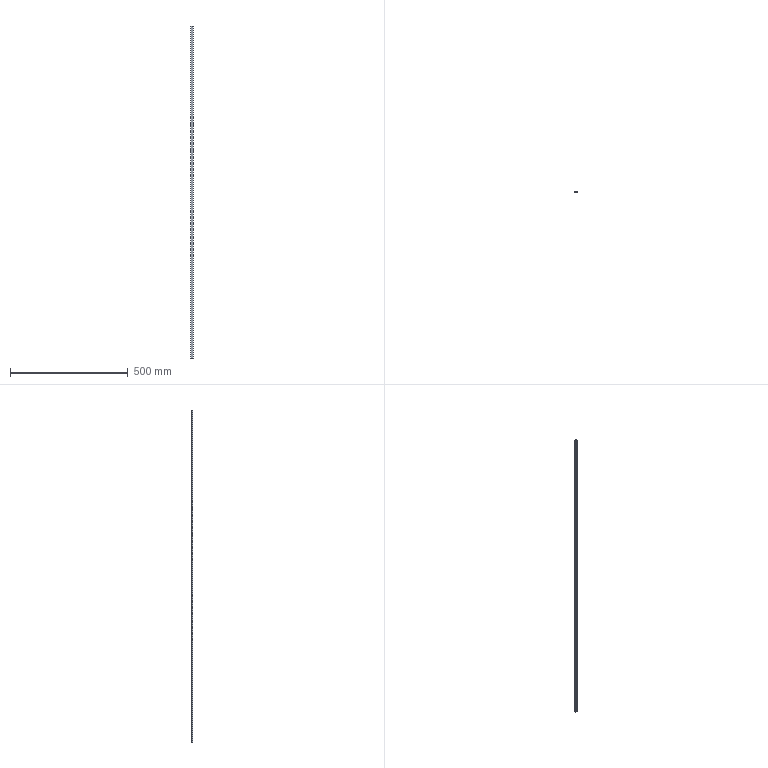Part | SolidWorks | features Extrusion 1 | 1 solid | 20 faces | box 10 x 6 x 1410 mm | volume 19879 mm3 | plane 12 | cylinder 8 | commonest cylinder face diameters 1 x3 2 x3 11.891 x1 12.891 x1
STEP:
#1=CARTESIAN_POINT('',(-4.13,5.131,705.));
#2=VERTEX_POINT('',#1);
#3=CARTESIAN_POINT('',(-4.283,4.771,705.));
#4=VERTEX_POINT('',#3);
#5=CARTESIAN_POINT('',(-3.783,4.771,705.));
#6=DIRECTION('',(0.,0.,1.));
#7=DIRECTION('',(1.,0.,0.));
#8=AXIS2_PLACEMENT_3D('',#5,#6,#7);
#9=CIRCLE('',#8,0.5);
#10=EDGE_CURVE('',#2,#4,#9,.T.);
#11=ORIENTED_EDGE('',*,*,#10,.T.);
#12=CARTESIAN_POINT('',(-4.283,4.771,-705.));
#13=VERTEX_POINT('',#12);
#14=CARTESIAN_POINT('',(-4.283,4.771,705.));
#15=DIRECTION('',(0.,0.,-1.));
#16=VECTOR('',#15,1000.);
#17=LINE('',#14,#16);
#18=EDGE_CURVE('',#4,#13,#17,.T.);
#19=ORIENTED_EDGE('',*,*,#18,.T.);
#20=CARTESIAN_POINT('',(-4.13,5.131,-705.));
#21=VERTEX_POINT('',#20);
#22=CARTESIAN_POINT('',(-3.783,4.771,-705.));
#23=DIRECTION('',(0.,0.,1.));
#24=DIRECTION('',(1.,0.,0.));
#25=AXIS2_PLACEMENT_3D('',#22,#23,#24);
#26=CIRCLE('',#25,0.5);
#27=EDGE_CURVE('',#21,#13,#26,.T.);
#28=ORIENTED_EDGE('',*,*,#27,.F.);
#29=CARTESIAN_POINT('',(-4.13,5.131,705.));
#30=DIRECTION('',(0.,0.,-1.));
#31=VECTOR('',#30,1000.);
#32=LINE('',#29,#31);
#33=EDGE_CURVE('',#2,#21,#32,.T.);
#34=ORIENTED_EDGE('',*,*,#33,.F.);
#35=EDGE_LOOP('',(#11,#19,#28,#34));
#36=FACE_OUTER_BOUND('',#35,.T.);
#37=CARTESIAN_POINT('',(-3.783,4.771,705.));
#38=DIRECTION('',(0.,0.,-1.));
#39=DIRECTION('',(-1.,0.,0.));
#40=AXIS2_PLACEMENT_3D('',#37,#38,#39);
#41=CYLINDRICAL_SURFACE('',#40,0.5);
#42=ADVANCED_FACE('',(#36),#41,.F.);
#43=CARTESIAN_POINT('',(-4.783,4.771,705.));
#44=VERTEX_POINT('',#43);
#45=CARTESIAN_POINT('',(-4.557,4.138,705.));
#46=VERTEX_POINT('',#45);
#47=CARTESIAN_POINT('',(-3.783,4.771,705.));
#48=DIRECTION('',(0.,0.,1.));
#49=DIRECTION('',(1.,0.,0.));
#50=AXIS2_PLACEMENT_3D('',#47,#48,#49);
#51=CIRCLE('',#50,1.);
#52=EDGE_CURVE('',#44,#46,#51,.T.);
#53=ORIENTED_EDGE('',*,*,#52,.F.);
#54=CARTESIAN_POINT('',(-4.783,4.771,-705.));
#55=VERTEX_POINT('',#54);
#56=CARTESIAN_POINT('',(-4.783,4.771,705.));
#57=DIRECTION('',(0.,0.,-1.));
#58=VECTOR('',#57,1000.);
#59=LINE('',#56,#58);
#60=EDGE_CURVE('',#44,#55,#59,.T.);
#61=ORIENTED_EDGE('',*,*,#60,.T.);
#62=CARTESIAN_POINT('',(-4.557,4.138,-705.));
#63=VERTEX_POINT('',#62);
#64=CARTESIAN_POINT('',(-3.783,4.771,-705.));
#65=DIRECTION('',(0.,0.,1.));
#66=DIRECTION('',(1.,0.,0.));
#67=AXIS2_PLACEMENT_3D('',#64,#65,#66);
#68=CIRCLE('',#67,1.);
#69=EDGE_CURVE('',#55,#63,#68,.T.);
#70=ORIENTED_EDGE('',*,*,#69,.T.);
#71=CARTESIAN_POINT('',(-4.557,4.138,705.));
#72=DIRECTION('',(0.,0.,-1.));
#73=VECTOR('',#72,1000.);
#74=LINE('',#71,#73);
#75=EDGE_CURVE('',#46,#63,#74,.T.);
#76=ORIENTED_EDGE('',*,*,#75,.F.);
#77=EDGE_LOOP('',(#53,#61,#70,#76));
#78=FACE_OUTER_BOUND('',#77,.T.);
#79=CARTESIAN_POINT('',(-3.783,4.771,705.));
#80=DIRECTION('',(0.,0.,-1.));
#81=DIRECTION('',(-1.,0.,0.));
#82=AXIS2_PLACEMENT_3D('',#79,#80,#81);
#83=CYLINDRICAL_SURFACE('',#82,1.);
#84=ADVANCED_FACE('',(#78),#83,.T.);
#85=CARTESIAN_POINT('',(-2.646,1.799,705.));
#86=VERTEX_POINT('',#85);
#87=CARTESIAN_POINT('',(-5.,1.799,705.));
#88=VERTEX_POINT('',#87);
#89=CARTESIAN_POINT('',(-2.646,1.799,705.));
#90=DIRECTION('',(-1.,0.,0.));
#91=VECTOR('',#90,1000.);
#92=LINE('',#89,#91);
#93=EDGE_CURVE('',#86,#88,#92,.T.);
#94=ORIENTED_EDGE('',*,*,#93,.T.);
#95=CARTESIAN_POINT('',(-5.,1.299,705.));
#96=VERTEX_POINT('',#95);
#97=CARTESIAN_POINT('',(-5.,1.799,705.));
#98=DIRECTION('',(0.,-1.,0.));
#99=VECTOR('',#98,1000.);
#100=LINE('',#97,#99);
#101=EDGE_CURVE('',#88,#96,#100,.T.);
#102=ORIENTED_EDGE('',*,*,#101,.T.);
#103=CARTESIAN_POINT('',(5.,1.299,705.));
#104=VERTEX_POINT('',#103);
#105=CARTESIAN_POINT('',(1.591,1.299,705.));
#106=DIRECTION('',(1.,0.,0.));
#107=VECTOR('',#106,1000.);
#108=LINE('',#105,#107);
#109=EDGE_CURVE('',#96,#104,#108,.T.);
#110=ORIENTED_EDGE('',*,*,#109,.T.);
#111=CARTESIAN_POINT('',(5.,1.799,705.));
#112=VERTEX_POINT('',#111);
#113=CARTESIAN_POINT('',(5.,1.799,705.));
#114=DIRECTION('',(0.,1.,0.));
#115=VECTOR('',#114,1000.);
#116=LINE('',#113,#115);
#117=EDGE_CURVE('',#104,#112,#116,.T.);
#118=ORIENTED_EDGE('',*,*,#117,.T.);
#119=CARTESIAN_POINT('',(2.646,1.799,705.));
#120=VERTEX_POINT('',#119);
#121=CARTESIAN_POINT('',(2.646,1.799,705.));
#122=DIRECTION('',(-1.,0.,0.));
#123=VECTOR('',#122,1000.);
#124=LINE('',#121,#123);
#125=EDGE_CURVE('',#112,#120,#124,.T.);
#126=ORIENTED_EDGE('',*,*,#125,.T.);
#127=CARTESIAN_POINT('',(4.557,4.138,705.));
#128=VERTEX_POINT('',#127);
#129=CARTESIAN_POINT('',(4.557,4.138,705.));
#130=DIRECTION('',(0.6327,0.7744,0.));
#131=VECTOR('',#130,1000.);
#132=LINE('',#129,#131);
#133=EDGE_CURVE('',#120,#128,#132,.T.);
#134=ORIENTED_EDGE('',*,*,#133,.T.);
#135=CARTESIAN_POINT('',(4.477,5.49,705.));
#136=VERTEX_POINT('',#135);
#137=CARTESIAN_POINT('',(3.783,4.771,705.));
#138=DIRECTION('',(0.,0.,1.));
#139=DIRECTION('',(-1.,0.,0.));
#140=AXIS2_PLACEMENT_3D('',#137,#138,#139);
#141=CIRCLE('',#140,1.);
#142=EDGE_CURVE('',#128,#136,#141,.T.);
#143=ORIENTED_EDGE('',*,*,#142,.T.);
#144=CARTESIAN_POINT('',(-4.477,5.49,705.));
#145=VERTEX_POINT('',#144);
#146=CARTESIAN_POINT('',(0.,0.8534,705.));
#147=DIRECTION('',(0.,0.,1.));
#148=DIRECTION('',(-1.,0.,0.));
#149=AXIS2_PLACEMENT_3D('',#146,#147,#148);
#150=CIRCLE('',#149,6.446);
#151=EDGE_CURVE('',#136,#145,#150,.T.);
#152=ORIENTED_EDGE('',*,*,#151,.T.);
#153=CARTESIAN_POINT('',(-3.783,4.771,705.));
#154=DIRECTION('',(0.,0.,1.));
#155=DIRECTION('',(1.,0.,0.));
#156=AXIS2_PLACEMENT_3D('',#153,#154,#155);
#157=CIRCLE('',#156,1.);
#158=EDGE_CURVE('',#145,#44,#157,.T.);
#159=ORIENTED_EDGE('',*,*,#158,.T.);
#160=ORIENTED_EDGE('',*,*,#52,.T.);
#161=CARTESIAN_POINT('',(-4.557,4.138,705.));
#162=DIRECTION('',(0.6327,-0.7744,0.));
#163=VECTOR('',#162,1000.);
#164=LINE('',#161,#163);
#165=EDGE_CURVE('',#46,#86,#164,.T.);
#166=ORIENTED_EDGE('',*,*,#165,.T.);
#167=EDGE_LOOP('',(#94,#102,#110,#118,#126,#134,#143,#152,#159,#160,#166));
#168=FACE_OUTER_BOUND('',#167,.T.);
#169=ORIENTED_EDGE('',*,*,#10,.F.);
#170=CARTESIAN_POINT('',(4.13,5.131,705.));
#171=VERTEX_POINT('',#170);
#172=CARTESIAN_POINT('',(0.,0.8534,705.));
#173=DIRECTION('',(0.,0.,1.));
#174=DIRECTION('',(-1.,0.,0.));
#175=AXIS2_PLACEMENT_3D('',#172,#173,#174);
#176=CIRCLE('',#175,5.946);
#177=EDGE_CURVE('',#171,#2,#176,.T.);
#178=ORIENTED_EDGE('',*,*,#177,.F.);
#179=CARTESIAN_POINT('',(4.17,4.454,705.));
#180=VERTEX_POINT('',#179);
#181=CARTESIAN_POINT('',(3.783,4.771,705.));
#182=DIRECTION('',(0.,0.,1.));
#183=DIRECTION('',(-1.,0.,0.));
#184=AXIS2_PLACEMENT_3D('',#181,#182,#183);
#185=CIRCLE('',#184,0.5);
#186=EDGE_CURVE('',#180,#171,#185,.T.);
#187=ORIENTED_EDGE('',*,*,#186,.F.);
#188=CARTESIAN_POINT('',(2.,1.799,705.));
#189=VERTEX_POINT('',#188);
#190=CARTESIAN_POINT('',(4.17,4.454,705.));
#191=DIRECTION('',(0.6327,0.7744,0.));
#192=VECTOR('',#191,1000.);
#193=LINE('',#190,#192);
#194=EDGE_CURVE('',#189,#180,#193,.T.);
#195=ORIENTED_EDGE('',*,*,#194,.F.);
#196=CARTESIAN_POINT('',(-2.,1.799,705.));
#197=VERTEX_POINT('',#196);
#198=CARTESIAN_POINT('',(-2.,1.799,705.));
#199=DIRECTION('',(1.,0.,0.));
#200=VECTOR('',#199,1000.);
#201=LINE('',#198,#200);
#202=EDGE_CURVE('',#197,#189,#201,.T.);
#203=ORIENTED_EDGE('',*,*,#202,.F.);
#204=CARTESIAN_POINT('',(-4.17,4.454,705.));
#205=VERTEX_POINT('',#204);
#206=CARTESIAN_POINT('',(-4.17,4.454,705.));
#207=DIRECTION('',(0.6327,-0.7744,0.));
#208=VECTOR('',#207,1000.);
#209=LINE('',#206,#208);
#210=EDGE_CURVE('',#205,#197,#209,.T.);
#211=ORIENTED_EDGE('',*,*,#210,.F.);
#212=CARTESIAN_POINT('',(-3.783,4.771,705.));
#213=DIRECTION('',(0.,0.,1.));
#214=DIRECTION('',(1.,0.,0.));
#215=AXIS2_PLACEMENT_3D('',#212,#213,#214);
#216=CIRCLE('',#215,0.5);
#217=EDGE_CURVE('',#4,#205,#216,.T.);
#218=ORIENTED_EDGE('',*,*,#217,.F.);
#219=EDGE_LOOP('',(#169,#178,#187,#195,#203,#211,#218));
#220=FACE_BOUND('',#219,.T.);
#221=CARTESIAN_POINT('',(3.783,4.771,705.));
#222=DIRECTION('',(0.,0.,-1.));
#223=DIRECTION('',(-1.,0.,0.));
#224=AXIS2_PLACEMENT_3D('',#221,#222,#223);
#225=PLANE('',#224);
#226=ADVANCED_FACE('',(#168,#220),#225,.F.);
#227=CARTESIAN_POINT('',(-2.646,1.799,-705.));
#228=VERTEX_POINT('',#227);
#229=CARTESIAN_POINT('',(-5.,1.799,-705.));
#230=VERTEX_POINT('',#229);
#231=CARTESIAN_POINT('',(-2.646,1.799,-705.));
#232=DIRECTION('',(-1.,0.,0.));
#233=VECTOR('',#232,1000.);
#234=LINE('',#231,#233);
#235=EDGE_CURVE('',#228,#230,#234,.T.);
#236=ORIENTED_EDGE('',*,*,#235,.F.);
#237=CARTESIAN_POINT('',(-4.557,4.138,-705.));
#238=DIRECTION('',(0.6327,-0.7744,0.));
#239=VECTOR('',#238,1000.);
#240=LINE('',#237,#239);
#241=EDGE_CURVE('',#63,#228,#240,.T.);
#242=ORIENTED_EDGE('',*,*,#241,.F.);
#243=ORIENTED_EDGE('',*,*,#69,.F.);
#244=CARTESIAN_POINT('',(-4.477,5.49,-705.));
#245=VERTEX_POINT('',#244);
#246=CARTESIAN_POINT('',(-3.783,4.771,-705.));
#247=DIRECTION('',(0.,0.,1.));
#248=DIRECTION('',(1.,0.,0.));
#249=AXIS2_PLACEMENT_3D('',#246,#247,#248);
#250=CIRCLE('',#249,1.);
#251=EDGE_CURVE('',#245,#55,#250,.T.);
#252=ORIENTED_EDGE('',*,*,#251,.F.);
#253=CARTESIAN_POINT('',(4.477,5.49,-705.));
#254=VERTEX_POINT('',#253);
#255=CARTESIAN_POINT('',(0.,0.8534,-705.));
#256=DIRECTION('',(0.,0.,1.));
#257=DIRECTION('',(-1.,0.,0.));
#258=AXIS2_PLACEMENT_3D('',#255,#256,#257);
#259=CIRCLE('',#258,6.446);
#260=EDGE_CURVE('',#254,#245,#259,.T.);
#261=ORIENTED_EDGE('',*,*,#260,.F.);
#262=CARTESIAN_POINT('',(4.557,4.138,-705.));
#263=VERTEX_POINT('',#262);
#264=CARTESIAN_POINT('',(3.783,4.771,-705.));
#265=DIRECTION('',(0.,0.,1.));
#266=DIRECTION('',(-1.,0.,0.));
#267=AXIS2_PLACEMENT_3D('',#264,#265,#266);
#268=CIRCLE('',#267,1.);
#269=EDGE_CURVE('',#263,#254,#268,.T.);
#270=ORIENTED_EDGE('',*,*,#269,.F.);
#271=CARTESIAN_POINT('',(2.646,1.799,-705.));
#272=VERTEX_POINT('',#271);
#273=CARTESIAN_POINT('',(4.557,4.138,-705.));
#274=DIRECTION('',(0.6327,0.7744,0.));
#275=VECTOR('',#274,1000.);
#276=LINE('',#273,#275);
#277=EDGE_CURVE('',#272,#263,#276,.T.);
#278=ORIENTED_EDGE('',*,*,#277,.F.);
#279=CARTESIAN_POINT('',(5.,1.799,-705.));
#280=VERTEX_POINT('',#279);
#281=CARTESIAN_POINT('',(2.646,1.799,-705.));
#282=DIRECTION('',(-1.,0.,0.));
#283=VECTOR('',#282,1000.);
#284=LINE('',#281,#283);
#285=EDGE_CURVE('',#280,#272,#284,.T.);
#286=ORIENTED_EDGE('',*,*,#285,.F.);
#287=CARTESIAN_POINT('',(5.,1.299,-705.));
#288=VERTEX_POINT('',#287);
#289=CARTESIAN_POINT('',(5.,1.799,-705.));
#290=DIRECTION('',(0.,1.,0.));
#291=VECTOR('',#290,1000.);
#292=LINE('',#289,#291);
#293=EDGE_CURVE('',#288,#280,#292,.T.);
#294=ORIENTED_EDGE('',*,*,#293,.F.);
#295=CARTESIAN_POINT('',(-5.,1.299,-705.));
#296=VERTEX_POINT('',#295);
#297=CARTESIAN_POINT('',(1.591,1.299,-705.));
#298=DIRECTION('',(1.,0.,0.));
#299=VECTOR('',#298,1000.);
#300=LINE('',#297,#299);
#301=EDGE_CURVE('',#296,#288,#300,.T.);
#302=ORIENTED_EDGE('',*,*,#301,.F.);
#303=CARTESIAN_POINT('',(-5.,1.799,-705.));
#304=DIRECTION('',(0.,-1.,0.));
#305=VECTOR('',#304,1000.);
#306=LINE('',#303,#305);
#307=EDGE_CURVE('',#230,#296,#306,.T.);
#308=ORIENTED_EDGE('',*,*,#307,.F.);
#309=EDGE_LOOP('',(#236,#242,#243,#252,#261,#270,#278,#286,#294,#302,#308));
#310=FACE_OUTER_BOUND('',#309,.T.);
#311=CARTESIAN_POINT('',(4.13,5.131,-705.));
#312=VERTEX_POINT('',#311);
#313=CARTESIAN_POINT('',(0.,0.8534,-705.));
#314=DIRECTION('',(0.,0.,1.));
#315=DIRECTION('',(-1.,0.,0.));
#316=AXIS2_PLACEMENT_3D('',#313,#314,#315);
#317=CIRCLE('',#316,5.946);
#318=EDGE_CURVE('',#312,#21,#317,.T.);
#319=ORIENTED_EDGE('',*,*,#318,.T.);
#320=ORIENTED_EDGE('',*,*,#27,.T.);
#321=CARTESIAN_POINT('',(-4.17,4.454,-705.));
#322=VERTEX_POINT('',#321);
#323=CARTESIAN_POINT('',(-3.783,4.771,-705.));
#324=DIRECTION('',(0.,0.,1.));
#325=DIRECTION('',(1.,0.,0.));
#326=AXIS2_PLACEMENT_3D('',#323,#324,#325);
#327=CIRCLE('',#326,0.5);
#328=EDGE_CURVE('',#13,#322,#327,.T.);
#329=ORIENTED_EDGE('',*,*,#328,.T.);
#330=CARTESIAN_POINT('',(-2.,1.799,-705.));
#331=VERTEX_POINT('',#330);
#332=CARTESIAN_POINT('',(-4.17,4.454,-705.));
#333=DIRECTION('',(0.6327,-0.7744,0.));
#334=VECTOR('',#333,1000.);
#335=LINE('',#332,#334);
#336=EDGE_CURVE('',#322,#331,#335,.T.);
#337=ORIENTED_EDGE('',*,*,#336,.T.);
#338=CARTESIAN_POINT('',(2.,1.799,-705.));
#339=VERTEX_POINT('',#338);
#340=CARTESIAN_POINT('',(-2.,1.799,-705.));
#341=DIRECTION('',(1.,0.,0.));
#342=VECTOR('',#341,1000.);
#343=LINE('',#340,#342);
#344=EDGE_CURVE('',#331,#339,#343,.T.);
#345=ORIENTED_EDGE('',*,*,#344,.T.);
#346=CARTESIAN_POINT('',(4.17,4.454,-705.));
#347=VERTEX_POINT('',#346);
#348=CARTESIAN_POINT('',(4.17,4.454,-705.));
#349=DIRECTION('',(0.6327,0.7744,0.));
#350=VECTOR('',#349,1000.);
#351=LINE('',#348,#350);
#352=EDGE_CURVE('',#339,#347,#351,.T.);
#353=ORIENTED_EDGE('',*,*,#352,.T.);
#354=CARTESIAN_POINT('',(3.783,4.771,-705.));
#355=DIRECTION('',(0.,0.,1.));
#356=DIRECTION('',(-1.,0.,0.));
#357=AXIS2_PLACEMENT_3D('',#354,#355,#356);
#358=CIRCLE('',#357,0.5);
#359=EDGE_CURVE('',#347,#312,#358,.T.);
#360=ORIENTED_EDGE('',*,*,#359,.T.);
#361=EDGE_LOOP('',(#319,#320,#329,#337,#345,#353,#360));
#362=FACE_BOUND('',#361,.T.);
#363=CARTESIAN_POINT('',(3.783,4.771,-705.));
#364=DIRECTION('',(0.,0.,-1.));
#365=DIRECTION('',(-1.,0.,0.));
#366=AXIS2_PLACEMENT_3D('',#363,#364,#365);
#367=PLANE('',#366);
#368=ADVANCED_FACE('',(#310,#362),#367,.T.);
#369=ORIENTED_EDGE('',*,*,#235,.T.);
#370=CARTESIAN_POINT('',(-5.,1.799,705.));
#371=DIRECTION('',(0.,0.,-1.));
#372=VECTOR('',#371,1000.);
#373=LINE('',#370,#372);
#374=EDGE_CURVE('',#88,#230,#373,.T.);
#375=ORIENTED_EDGE('',*,*,#374,.F.);
#376=ORIENTED_EDGE('',*,*,#93,.F.);
#377=CARTESIAN_POINT('',(-2.646,1.799,705.));
#378=DIRECTION('',(0.,0.,-1.));
#379=VECTOR('',#378,1000.);
#380=LINE('',#377,#379);
#381=EDGE_CURVE('',#86,#228,#380,.T.);
#382=ORIENTED_EDGE('',*,*,#381,.T.);
#383=EDGE_LOOP('',(#369,#375,#376,#382));
#384=FACE_OUTER_BOUND('',#383,.T.);
#385=CARTESIAN_POINT('',(-2.646,1.799,705.));
#386=DIRECTION('',(0.,-1.,0.));
#387=DIRECTION('',(1.,0.,0.));
#388=AXIS2_PLACEMENT_3D('',#385,#386,#387);
#389=PLANE('',#388);
#390=ADVANCED_FACE('',(#384),#389,.F.);
#391=ORIENTED_EDGE('',*,*,#307,.T.);
#392=CARTESIAN_POINT('',(-5.,1.299,705.));
#393=DIRECTION('',(0.,0.,-1.));
#394=VECTOR('',#393,1000.);
#395=LINE('',#392,#394);
#396=EDGE_CURVE('',#96,#296,#395,.T.);
#397=ORIENTED_EDGE('',*,*,#396,.F.);
#398=ORIENTED_EDGE('',*,*,#101,.F.);
#399=ORIENTED_EDGE('',*,*,#374,.T.);
#400=EDGE_LOOP('',(#391,#397,#398,#399));
#401=FACE_OUTER_BOUND('',#400,.T.);
#402=CARTESIAN_POINT('',(-5.,1.799,705.));
#403=DIRECTION('',(1.,0.,0.));
#404=DIRECTION('',(0.,0.,-1.));
#405=AXIS2_PLACEMENT_3D('',#402,#403,#404);
#406=PLANE('',#405);
#407=ADVANCED_FACE('',(#401),#406,.F.);
#408=ORIENTED_EDGE('',*,*,#301,.T.);
#409=CARTESIAN_POINT('',(5.,1.299,705.));
#410=DIRECTION('',(0.,0.,-1.));
#411=VECTOR('',#410,1000.);
#412=LINE('',#409,#411);
#413=EDGE_CURVE('',#104,#288,#412,.T.);
#414=ORIENTED_EDGE('',*,*,#413,.F.);
#415=ORIENTED_EDGE('',*,*,#109,.F.);
#416=ORIENTED_EDGE('',*,*,#396,.T.);
#417=EDGE_LOOP('',(#408,#414,#415,#416));
#418=FACE_OUTER_BOUND('',#417,.T.);
#419=CARTESIAN_POINT('',(1.591,1.299,705.));
#420=DIRECTION('',(0.,1.,0.));
#421=DIRECTION('',(-1.,0.,0.));
#422=AXIS2_PLACEMENT_3D('',#419,#420,#421);
#423=PLANE('',#422);
#424=ADVANCED_FACE('',(#418),#423,.F.);
#425=ORIENTED_EDGE('',*,*,#293,.T.);
#426=CARTESIAN_POINT('',(5.,1.799,705.));
#427=DIRECTION('',(0.,0.,-1.));
#428=VECTOR('',#427,1000.);
#429=LINE('',#426,#428);
#430=EDGE_CURVE('',#112,#280,#429,.T.);
#431=ORIENTED_EDGE('',*,*,#430,.F.);
#432=ORIENTED_EDGE('',*,*,#117,.F.);
#433=ORIENTED_EDGE('',*,*,#413,.T.);
#434=EDGE_LOOP('',(#425,#431,#432,#433));
#435=FACE_OUTER_BOUND('',#434,.T.);
#436=CARTESIAN_POINT('',(5.,1.799,705.));
#437=DIRECTION('',(-1.,0.,0.));
#438=DIRECTION('',(0.,0.,1.));
#439=AXIS2_PLACEMENT_3D('',#436,#437,#438);
#440=PLANE('',#439);
#441=ADVANCED_FACE('',(#435),#440,.F.);
#442=ORIENTED_EDGE('',*,*,#285,.T.);
#443=CARTESIAN_POINT('',(2.646,1.799,705.));
#444=DIRECTION('',(0.,0.,-1.));
#445=VECTOR('',#444,1000.);
#446=LINE('',#443,#445);
#447=EDGE_CURVE('',#120,#272,#446,.T.);
#448=ORIENTED_EDGE('',*,*,#447,.F.);
#449=ORIENTED_EDGE('',*,*,#125,.F.);
#450=ORIENTED_EDGE('',*,*,#430,.T.);
#451=EDGE_LOOP('',(#442,#448,#449,#450));
#452=FACE_OUTER_BOUND('',#451,.T.);
#453=CARTESIAN_POINT('',(2.646,1.799,705.));
#454=DIRECTION('',(0.,-1.,0.));
#455=DIRECTION('',(1.,0.,0.));
#456=AXIS2_PLACEMENT_3D('',#453,#454,#455);
#457=PLANE('',#456);
#458=ADVANCED_FACE('',(#452),#457,.F.);
#459=ORIENTED_EDGE('',*,*,#277,.T.);
#460=CARTESIAN_POINT('',(4.557,4.138,705.));
#461=DIRECTION('',(0.,0.,-1.));
#462=VECTOR('',#461,1000.);
#463=LINE('',#460,#462);
#464=EDGE_CURVE('',#128,#263,#463,.T.);
#465=ORIENTED_EDGE('',*,*,#464,.F.);
#466=ORIENTED_EDGE('',*,*,#133,.F.);
#467=ORIENTED_EDGE('',*,*,#447,.T.);
#468=EDGE_LOOP('',(#459,#465,#466,#467));
#469=FACE_OUTER_BOUND('',#468,.T.);
#470=CARTESIAN_POINT('',(4.557,4.138,705.));
#471=DIRECTION('',(-0.7744,0.6327,0.));
#472=DIRECTION('',(-0.6327,-0.7744,0.));
#473=AXIS2_PLACEMENT_3D('',#470,#471,#472);
#474=PLANE('',#473);
#475=ADVANCED_FACE('',(#469),#474,.F.);
#476=ORIENTED_EDGE('',*,*,#269,.T.);
#477=CARTESIAN_POINT('',(4.477,5.49,705.));
#478=DIRECTION('',(0.,0.,-1.));
#479=VECTOR('',#478,1000.);
#480=LINE('',#477,#479);
#481=EDGE_CURVE('',#136,#254,#480,.T.);
#482=ORIENTED_EDGE('',*,*,#481,.F.);
#483=ORIENTED_EDGE('',*,*,#142,.F.);
#484=ORIENTED_EDGE('',*,*,#464,.T.);
#485=EDGE_LOOP('',(#476,#482,#483,#484));
#486=FACE_OUTER_BOUND('',#485,.T.);
#487=CARTESIAN_POINT('',(3.783,4.771,705.));
#488=DIRECTION('',(0.,0.,-1.));
#489=DIRECTION('',(-1.,0.,0.));
#490=AXIS2_PLACEMENT_3D('',#487,#488,#489);
#491=CYLINDRICAL_SURFACE('',#490,1.);
#492=ADVANCED_FACE('',(#486),#491,.T.);
#493=ORIENTED_EDGE('',*,*,#260,.T.);
#494=CARTESIAN_POINT('',(-4.477,5.49,705.));
#495=DIRECTION('',(0.,0.,-1.));
#496=VECTOR('',#495,1000.);
#497=LINE('',#494,#496);
#498=EDGE_CURVE('',#145,#245,#497,.T.);
#499=ORIENTED_EDGE('',*,*,#498,.F.);
#500=ORIENTED_EDGE('',*,*,#151,.F.);
#501=ORIENTED_EDGE('',*,*,#481,.T.);
#502=EDGE_LOOP('',(#493,#499,#500,#501));
#503=FACE_OUTER_BOUND('',#502,.T.);
#504=CARTESIAN_POINT('',(0.,0.8534,705.));
#505=DIRECTION('',(0.,0.,-1.));
#506=DIRECTION('',(-1.,0.,0.));
#507=AXIS2_PLACEMENT_3D('',#504,#505,#506);
#508=CYLINDRICAL_SURFACE('',#507,6.446);
#509=ADVANCED_FACE('',(#503),#508,.T.);
#510=ORIENTED_EDGE('',*,*,#60,.F.);
#511=ORIENTED_EDGE('',*,*,#158,.F.);
#512=ORIENTED_EDGE('',*,*,#498,.T.);
#513=ORIENTED_EDGE('',*,*,#251,.T.);
#514=EDGE_LOOP('',(#510,#511,#512,#513));
#515=FACE_OUTER_BOUND('',#514,.T.);
#516=CARTESIAN_POINT('',(-3.783,4.771,705.));
#517=DIRECTION('',(0.,0.,-1.));
#518=DIRECTION('',(-1.,0.,0.));
#519=AXIS2_PLACEMENT_3D('',#516,#517,#518);
#520=CYLINDRICAL_SURFACE('',#519,1.);
#521=ADVANCED_FACE('',(#515),#520,.T.);
#522=ORIENTED_EDGE('',*,*,#241,.T.);
#523=ORIENTED_EDGE('',*,*,#381,.F.);
#524=ORIENTED_EDGE('',*,*,#165,.F.);
#525=ORIENTED_EDGE('',*,*,#75,.T.);
#526=EDGE_LOOP('',(#522,#523,#524,#525));
#527=FACE_OUTER_BOUND('',#526,.T.);
#528=CARTESIAN_POINT('',(-4.557,4.138,705.));
#529=DIRECTION('',(0.7744,0.6327,0.));
#530=DIRECTION('',(-0.6327,0.7744,0.));
#531=AXIS2_PLACEMENT_3D('',#528,#529,#530);
#532=PLANE('',#531);
#533=ADVANCED_FACE('',(#527),#532,.F.);
#534=ORIENTED_EDGE('',*,*,#18,.F.);
#535=ORIENTED_EDGE('',*,*,#217,.T.);
#536=CARTESIAN_POINT('',(-4.17,4.454,705.));
#537=DIRECTION('',(0.,0.,-1.));
#538=VECTOR('',#537,1000.);
#539=LINE('',#536,#538);
#540=EDGE_CURVE('',#205,#322,#539,.T.);
#541=ORIENTED_EDGE('',*,*,#540,.T.);
#542=ORIENTED_EDGE('',*,*,#328,.F.);
#543=EDGE_LOOP('',(#534,#535,#541,#542));
#544=FACE_OUTER_BOUND('',#543,.T.);
#545=CARTESIAN_POINT('',(-3.783,4.771,705.));
#546=DIRECTION('',(0.,0.,-1.));
#547=DIRECTION('',(-1.,0.,0.));
#548=AXIS2_PLACEMENT_3D('',#545,#546,#547);
#549=CYLINDRICAL_SURFACE('',#548,0.5);
#550=ADVANCED_FACE('',(#544),#549,.F.);
#551=ORIENTED_EDGE('',*,*,#336,.F.);
#552=ORIENTED_EDGE('',*,*,#540,.F.);
#553=ORIENTED_EDGE('',*,*,#210,.T.);
#554=CARTESIAN_POINT('',(-2.,1.799,705.));
#555=DIRECTION('',(0.,0.,-1.));
#556=VECTOR('',#555,1000.);
#557=LINE('',#554,#556);
#558=EDGE_CURVE('',#197,#331,#557,.T.);
#559=ORIENTED_EDGE('',*,*,#558,.T.);
#560=EDGE_LOOP('',(#551,#552,#553,#559));
#561=FACE_OUTER_BOUND('',#560,.T.);
#562=CARTESIAN_POINT('',(-4.17,4.454,705.));
#563=DIRECTION('',(0.7744,0.6327,0.));
#564=DIRECTION('',(-0.6327,0.7744,0.));
#565=AXIS2_PLACEMENT_3D('',#562,#563,#564);
#566=PLANE('',#565);
#567=ADVANCED_FACE('',(#561),#566,.T.);
#568=ORIENTED_EDGE('',*,*,#344,.F.);
#569=ORIENTED_EDGE('',*,*,#558,.F.);
#570=ORIENTED_EDGE('',*,*,#202,.T.);
#571=CARTESIAN_POINT('',(2.,1.799,705.));
#572=DIRECTION('',(0.,0.,-1.));
#573=VECTOR('',#572,1000.);
#574=LINE('',#571,#573);
#575=EDGE_CURVE('',#189,#339,#574,.T.);
#576=ORIENTED_EDGE('',*,*,#575,.T.);
#577=EDGE_LOOP('',(#568,#569,#570,#576));
#578=FACE_OUTER_BOUND('',#577,.T.);
#579=CARTESIAN_POINT('',(-2.,1.799,705.));
#580=DIRECTION('',(0.,1.,0.));
#581=DIRECTION('',(0.,0.,1.));
#582=AXIS2_PLACEMENT_3D('',#579,#580,#581);
#583=PLANE('',#582);
#584=ADVANCED_FACE('',(#578),#583,.T.);
#585=ORIENTED_EDGE('',*,*,#352,.F.);
#586=ORIENTED_EDGE('',*,*,#575,.F.);
#587=ORIENTED_EDGE('',*,*,#194,.T.);
#588=CARTESIAN_POINT('',(4.17,4.454,705.));
#589=DIRECTION('',(0.,0.,-1.));
#590=VECTOR('',#589,1000.);
#591=LINE('',#588,#590);
#592=EDGE_CURVE('',#180,#347,#591,.T.);
#593=ORIENTED_EDGE('',*,*,#592,.T.);
#594=EDGE_LOOP('',(#585,#586,#587,#593));
#595=FACE_OUTER_BOUND('',#594,.T.);
#596=CARTESIAN_POINT('',(4.17,4.454,705.));
#597=DIRECTION('',(-0.7744,0.6327,0.));
#598=DIRECTION('',(-0.6327,-0.7744,0.));
#599=AXIS2_PLACEMENT_3D('',#596,#597,#598);
#600=PLANE('',#599);
#601=ADVANCED_FACE('',(#595),#600,.T.);
#602=ORIENTED_EDGE('',*,*,#359,.F.);
#603=ORIENTED_EDGE('',*,*,#592,.F.);
#604=ORIENTED_EDGE('',*,*,#186,.T.);
#605=CARTESIAN_POINT('',(4.13,5.131,705.));
#606=DIRECTION('',(0.,0.,-1.));
#607=VECTOR('',#606,1000.);
#608=LINE('',#605,#607);
#609=EDGE_CURVE('',#171,#312,#608,.T.);
#610=ORIENTED_EDGE('',*,*,#609,.T.);
#611=EDGE_LOOP('',(#602,#603,#604,#610));
#612=FACE_OUTER_BOUND('',#611,.T.);
#613=CARTESIAN_POINT('',(3.783,4.771,705.));
#614=DIRECTION('',(0.,0.,-1.));
#615=DIRECTION('',(-1.,0.,0.));
#616=AXIS2_PLACEMENT_3D('',#613,#614,#615);
#617=CYLINDRICAL_SURFACE('',#616,0.5);
#618=ADVANCED_FACE('',(#612),#617,.F.);
#619=ORIENTED_EDGE('',*,*,#318,.F.);
#620=ORIENTED_EDGE('',*,*,#609,.F.);
#621=ORIENTED_EDGE('',*,*,#177,.T.);
#622=ORIENTED_EDGE('',*,*,#33,.T.);
#623=EDGE_LOOP('',(#619,#620,#621,#622));
#624=FACE_OUTER_BOUND('',#623,.T.);
#625=CARTESIAN_POINT('',(0.,0.8534,705.));
#626=DIRECTION('',(0.,0.,-1.));
#627=DIRECTION('',(-1.,0.,0.));
#628=AXIS2_PLACEMENT_3D('',#625,#626,#627);
#629=CYLINDRICAL_SURFACE('',#628,5.946);
#630=ADVANCED_FACE('',(#624),#629,.F.);
#631=CLOSED_SHELL('',(#42,#84,#226,#368,#390,#407,#424,#441,#458,#475,#492,#509,#521,#533,#550,#567,#584,#601,#618,#630));
#632=MANIFOLD_SOLID_BREP('',#631);
#633=CARTESIAN_POINT('',(0.,0.,0.));
#634=DIRECTION('',(0.,0.,1.));
#635=DIRECTION('',(1.,0.,0.));
#636=AXIS2_PLACEMENT_3D('',#633,#634,#635);
#637=(LENGTH_UNIT()NAMED_UNIT(*)SI_UNIT(.MILLI.,.METRE.));
#638=UNCERTAINTY_MEASURE_WITH_UNIT(LENGTH_MEASURE(0.00001),#637,'','');
#639=(NAMED_UNIT(*)PLANE_ANGLE_UNIT()SI_UNIT($,.RADIAN.));
#640=(NAMED_UNIT(*)SI_UNIT($,.STERADIAN.)SOLID_ANGLE_UNIT());
#641=(GEOMETRIC_REPRESENTATION_CONTEXT(3)GLOBAL_UNCERTAINTY_ASSIGNED_CONTEXT((#638))GLOBAL_UNIT_ASSIGNED_CONTEXT((#637,#639,#640))REPRESENTATION_CONTEXT('',''));
#642=ADVANCED_BREP_SHAPE_REPRESENTATION('',(#632,#636),#641);